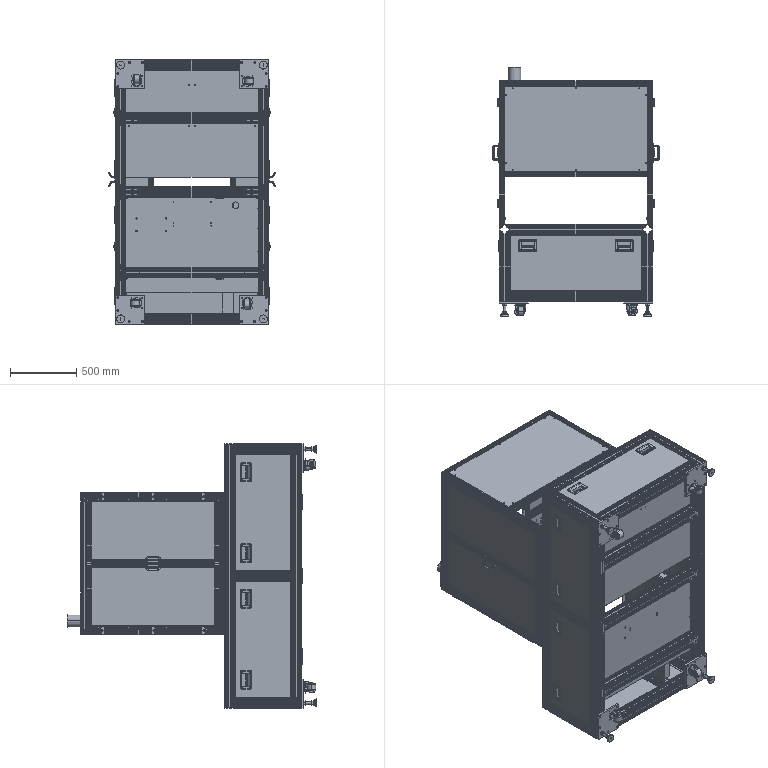Part | SolidWorks | 289 solids | 14057 faces | volume 99819885 mm3 | plane 8488 | cylinder 4922 | cone 491 | torus 128 | sphere 20 | spline 8 | commonest cylinder face diameters 2 x732 5 x520 0.6 x382 7 x380 6 x280 6.8 x272